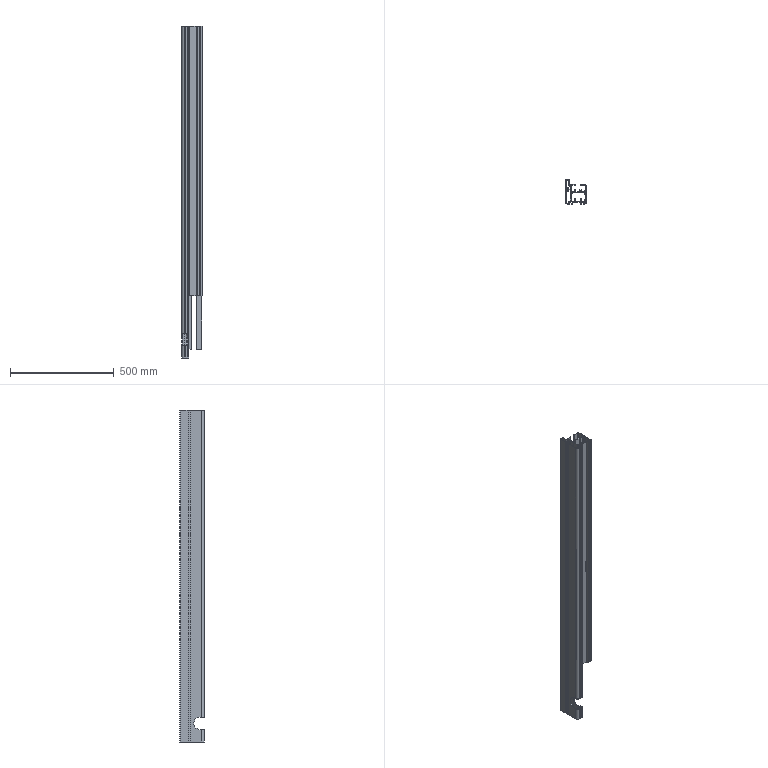Part | STEP file | 1 solid | 242 faces | box 100 x 118 x 1600 mm | volume 2582568 mm3 | plane 144 | cylinder 98 | commonest cylinder face diameters 1 x65 4 x23 2 x2 20 x2 24 x2 60 x2